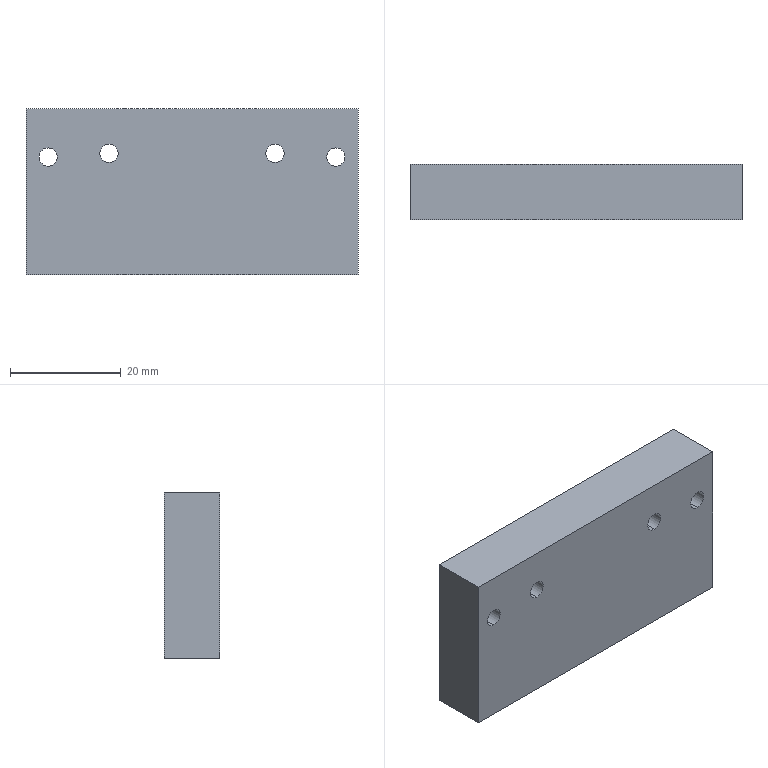Part | STEP file | 227H056123 Block_Default | 1 solid | 14 faces | box 60 x 10 x 30 mm | volume 17658 mm3 | cylinder 8 | plane 6 | commonest cylinder face diameters 3.3 x8
STEP:
#1=CARTESIAN_POINT('',(0.,0.,0.));
#2=DIRECTION('',(0.,0.,1.));
#3=DIRECTION('',(1.,0.,0.));
#4=AXIS2_PLACEMENT_3D('',#1,#2,#3);
#5=CARTESIAN_POINT('',(15.,0.,8.65));
#6=VERTEX_POINT('',#5);
#7=CARTESIAN_POINT('',(15.,10.,8.65));
#8=VERTEX_POINT('',#7);
#9=CARTESIAN_POINT('',(15.,10.,8.65));
#10=DIRECTION('',(0.,1.,0.));
#11=VECTOR('',#10,1.);
#12=LINE('',#9,#11);
#13=CARTESIAN_POINT('',(15.,10.,7.));
#14=DIRECTION('',(0.,1.,0.));
#15=DIRECTION('',(0.,0.,1.));
#16=AXIS2_PLACEMENT_3D('',#13,#14,#15);
#17=CYLINDRICAL_SURFACE('',#16,1.65);
#18=CARTESIAN_POINT('',(6.283,0.));
#19=DIRECTION('',(0.,1.));
#20=VECTOR('',#19,1.);
#21=LINE('',#18,#20);
#22=(GEOMETRIC_REPRESENTATION_CONTEXT(2)PARAMETRIC_REPRESENTATION_CONTEXT()REPRESENTATION_CONTEXT('',''));
#23=DEFINITIONAL_REPRESENTATION('',(#21),#22);
#24=PCURVE('',#17,#23);
#25=CARTESIAN_POINT('',(15.,10.,7.));
#26=DIRECTION('',(0.,1.,0.));
#27=DIRECTION('',(0.,0.,1.));
#28=AXIS2_PLACEMENT_3D('',#25,#26,#27);
#29=CYLINDRICAL_SURFACE('',#28,1.65);
#30=CARTESIAN_POINT('',(0.,0.));
#31=DIRECTION('',(0.,1.));
#32=VECTOR('',#31,1.);
#33=LINE('',#30,#32);
#34=(GEOMETRIC_REPRESENTATION_CONTEXT(2)PARAMETRIC_REPRESENTATION_CONTEXT()REPRESENTATION_CONTEXT('',''));
#35=DEFINITIONAL_REPRESENTATION('',(#33),#34);
#36=PCURVE('',#29,#35);
#37=SURFACE_CURVE('',#12,(#24,#36),.PCURVE_S1.);
#38=EDGE_CURVE('',#6,#8,#37,.T.);
#39=ORIENTED_EDGE('',*,*,#38,.T.);
#40=CARTESIAN_POINT('',(15.,10.,5.35));
#41=VERTEX_POINT('',#40);
#42=CARTESIAN_POINT('',(15.,10.,7.));
#43=DIRECTION('',(0.,1.,0.));
#44=DIRECTION('',(0.,0.,1.));
#45=AXIS2_PLACEMENT_3D('',#42,#43,#44);
#46=CIRCLE('',#45,1.65);
#47=CARTESIAN_POINT('',(0.,0.));
#48=DIRECTION('',(1.,0.));
#49=VECTOR('',#48,1.);
#50=LINE('',#47,#49);
#51=(GEOMETRIC_REPRESENTATION_CONTEXT(2)PARAMETRIC_REPRESENTATION_CONTEXT()REPRESENTATION_CONTEXT('',''));
#52=DEFINITIONAL_REPRESENTATION('',(#50),#51);
#53=PCURVE('',#17,#52);
#54=CARTESIAN_POINT('',(0.,10.,0.));
#55=DIRECTION('',(0.,1.,0.));
#56=DIRECTION('',(0.,0.,1.));
#57=AXIS2_PLACEMENT_3D('',#54,#55,#56);
#58=PLANE('',#57);
#59=CARTESIAN_POINT('',(7.,15.));
#60=DIRECTION('',(1.,0.));
#61=AXIS2_PLACEMENT_2D('',#59,#60);
#62=CIRCLE('',#61,1.65);
#63=(GEOMETRIC_REPRESENTATION_CONTEXT(2)PARAMETRIC_REPRESENTATION_CONTEXT()REPRESENTATION_CONTEXT('',''));
#64=DEFINITIONAL_REPRESENTATION('',(#62),#63);
#65=PCURVE('',#58,#64);
#66=SURFACE_CURVE('',#46,(#53,#65),.PCURVE_S1.);
#67=EDGE_CURVE('',#41,#8,#66,.T.);
#68=ORIENTED_EDGE('',*,*,#67,.F.);
#69=CARTESIAN_POINT('',(15.,0.,5.35));
#70=VERTEX_POINT('',#69);
#71=CARTESIAN_POINT('',(15.,10.,5.35));
#72=DIRECTION('',(0.,1.,0.));
#73=VECTOR('',#72,1.);
#74=LINE('',#71,#73);
#75=CARTESIAN_POINT('',(3.142,0.));
#76=DIRECTION('',(0.,1.));
#77=VECTOR('',#76,1.);
#78=LINE('',#75,#77);
#79=(GEOMETRIC_REPRESENTATION_CONTEXT(2)PARAMETRIC_REPRESENTATION_CONTEXT()REPRESENTATION_CONTEXT('',''));
#80=DEFINITIONAL_REPRESENTATION('',(#78),#79);
#81=PCURVE('',#17,#80);
#82=CARTESIAN_POINT('',(3.142,0.));
#83=DIRECTION('',(0.,1.));
#84=VECTOR('',#83,1.);
#85=LINE('',#82,#84);
#86=(GEOMETRIC_REPRESENTATION_CONTEXT(2)PARAMETRIC_REPRESENTATION_CONTEXT()REPRESENTATION_CONTEXT('',''));
#87=DEFINITIONAL_REPRESENTATION('',(#85),#86);
#88=PCURVE('',#29,#87);
#89=SURFACE_CURVE('',#74,(#81,#88),.PCURVE_S1.);
#90=EDGE_CURVE('',#70,#41,#89,.T.);
#91=ORIENTED_EDGE('',*,*,#90,.F.);
#92=CARTESIAN_POINT('',(15.,0.,7.));
#93=DIRECTION('',(0.,1.,0.));
#94=DIRECTION('',(0.,0.,1.));
#95=AXIS2_PLACEMENT_3D('',#92,#93,#94);
#96=CIRCLE('',#95,1.65);
#97=CARTESIAN_POINT('',(0.,-10.));
#98=DIRECTION('',(1.,0.));
#99=VECTOR('',#98,1.);
#100=LINE('',#97,#99);
#101=(GEOMETRIC_REPRESENTATION_CONTEXT(2)PARAMETRIC_REPRESENTATION_CONTEXT()REPRESENTATION_CONTEXT('',''));
#102=DEFINITIONAL_REPRESENTATION('',(#100),#101);
#103=PCURVE('',#17,#102);
#104=CARTESIAN_POINT('',(0.,0.,0.));
#105=DIRECTION('',(0.,1.,0.));
#106=DIRECTION('',(0.,0.,1.));
#107=AXIS2_PLACEMENT_3D('',#104,#105,#106);
#108=PLANE('',#107);
#109=CARTESIAN_POINT('',(7.,15.));
#110=DIRECTION('',(1.,0.));
#111=AXIS2_PLACEMENT_2D('',#109,#110);
#112=CIRCLE('',#111,1.65);
#113=(GEOMETRIC_REPRESENTATION_CONTEXT(2)PARAMETRIC_REPRESENTATION_CONTEXT()REPRESENTATION_CONTEXT('',''));
#114=DEFINITIONAL_REPRESENTATION('',(#112),#113);
#115=PCURVE('',#108,#114);
#116=SURFACE_CURVE('',#96,(#103,#115),.PCURVE_S1.);
#117=EDGE_CURVE('',#70,#6,#116,.T.);
#118=ORIENTED_EDGE('',*,*,#117,.T.);
#119=EDGE_LOOP('',(#39,#68,#91,#118));
#120=FACE_BOUND('',#119,.F.);
#121=ADVANCED_FACE('',(#120),#17,.F.);
#122=CARTESIAN_POINT('',(-15.,0.,8.65));
#123=VERTEX_POINT('',#122);
#124=CARTESIAN_POINT('',(-15.,10.,8.65));
#125=VERTEX_POINT('',#124);
#126=CARTESIAN_POINT('',(-15.,10.,8.65));
#127=DIRECTION('',(0.,1.,0.));
#128=VECTOR('',#127,1.);
#129=LINE('',#126,#128);
#130=CARTESIAN_POINT('',(-15.,10.,7.));
#131=DIRECTION('',(0.,1.,0.));
#132=DIRECTION('',(0.,0.,1.));
#133=AXIS2_PLACEMENT_3D('',#130,#131,#132);
#134=CYLINDRICAL_SURFACE('',#133,1.65);
#135=CARTESIAN_POINT('',(6.283,0.));
#136=DIRECTION('',(0.,1.));
#137=VECTOR('',#136,1.);
#138=LINE('',#135,#137);
#139=(GEOMETRIC_REPRESENTATION_CONTEXT(2)PARAMETRIC_REPRESENTATION_CONTEXT()REPRESENTATION_CONTEXT('',''));
#140=DEFINITIONAL_REPRESENTATION('',(#138),#139);
#141=PCURVE('',#134,#140);
#142=CARTESIAN_POINT('',(-15.,10.,7.));
#143=DIRECTION('',(0.,1.,0.));
#144=DIRECTION('',(0.,0.,1.));
#145=AXIS2_PLACEMENT_3D('',#142,#143,#144);
#146=CYLINDRICAL_SURFACE('',#145,1.65);
#147=CARTESIAN_POINT('',(0.,0.));
#148=DIRECTION('',(0.,1.));
#149=VECTOR('',#148,1.);
#150=LINE('',#147,#149);
#151=(GEOMETRIC_REPRESENTATION_CONTEXT(2)PARAMETRIC_REPRESENTATION_CONTEXT()REPRESENTATION_CONTEXT('',''));
#152=DEFINITIONAL_REPRESENTATION('',(#150),#151);
#153=PCURVE('',#146,#152);
#154=SURFACE_CURVE('',#129,(#141,#153),.PCURVE_S1.);
#155=EDGE_CURVE('',#123,#125,#154,.T.);
#156=ORIENTED_EDGE('',*,*,#155,.T.);
#157=CARTESIAN_POINT('',(-15.,10.,5.35));
#158=VERTEX_POINT('',#157);
#159=CARTESIAN_POINT('',(-15.,10.,7.));
#160=DIRECTION('',(0.,1.,0.));
#161=DIRECTION('',(0.,0.,1.));
#162=AXIS2_PLACEMENT_3D('',#159,#160,#161);
#163=CIRCLE('',#162,1.65);
#164=CARTESIAN_POINT('',(0.,0.));
#165=DIRECTION('',(1.,0.));
#166=VECTOR('',#165,1.);
#167=LINE('',#164,#166);
#168=(GEOMETRIC_REPRESENTATION_CONTEXT(2)PARAMETRIC_REPRESENTATION_CONTEXT()REPRESENTATION_CONTEXT('',''));
#169=DEFINITIONAL_REPRESENTATION('',(#167),#168);
#170=PCURVE('',#134,#169);
#171=CARTESIAN_POINT('',(7.,-15.));
#172=DIRECTION('',(1.,0.));
#173=AXIS2_PLACEMENT_2D('',#171,#172);
#174=CIRCLE('',#173,1.65);
#175=(GEOMETRIC_REPRESENTATION_CONTEXT(2)PARAMETRIC_REPRESENTATION_CONTEXT()REPRESENTATION_CONTEXT('',''));
#176=DEFINITIONAL_REPRESENTATION('',(#174),#175);
#177=PCURVE('',#58,#176);
#178=SURFACE_CURVE('',#163,(#170,#177),.PCURVE_S1.);
#179=EDGE_CURVE('',#158,#125,#178,.T.);
#180=ORIENTED_EDGE('',*,*,#179,.F.);
#181=CARTESIAN_POINT('',(-15.,0.,5.35));
#182=VERTEX_POINT('',#181);
#183=CARTESIAN_POINT('',(-15.,10.,5.35));
#184=DIRECTION('',(0.,1.,0.));
#185=VECTOR('',#184,1.);
#186=LINE('',#183,#185);
#187=CARTESIAN_POINT('',(3.142,0.));
#188=DIRECTION('',(0.,1.));
#189=VECTOR('',#188,1.);
#190=LINE('',#187,#189);
#191=(GEOMETRIC_REPRESENTATION_CONTEXT(2)PARAMETRIC_REPRESENTATION_CONTEXT()REPRESENTATION_CONTEXT('',''));
#192=DEFINITIONAL_REPRESENTATION('',(#190),#191);
#193=PCURVE('',#134,#192);
#194=CARTESIAN_POINT('',(3.142,0.));
#195=DIRECTION('',(0.,1.));
#196=VECTOR('',#195,1.);
#197=LINE('',#194,#196);
#198=(GEOMETRIC_REPRESENTATION_CONTEXT(2)PARAMETRIC_REPRESENTATION_CONTEXT()REPRESENTATION_CONTEXT('',''));
#199=DEFINITIONAL_REPRESENTATION('',(#197),#198);
#200=PCURVE('',#146,#199);
#201=SURFACE_CURVE('',#186,(#193,#200),.PCURVE_S1.);
#202=EDGE_CURVE('',#182,#158,#201,.T.);
#203=ORIENTED_EDGE('',*,*,#202,.F.);
#204=CARTESIAN_POINT('',(-15.,0.,7.));
#205=DIRECTION('',(0.,1.,0.));
#206=DIRECTION('',(0.,0.,1.));
#207=AXIS2_PLACEMENT_3D('',#204,#205,#206);
#208=CIRCLE('',#207,1.65);
#209=CARTESIAN_POINT('',(0.,-10.));
#210=DIRECTION('',(1.,0.));
#211=VECTOR('',#210,1.);
#212=LINE('',#209,#211);
#213=(GEOMETRIC_REPRESENTATION_CONTEXT(2)PARAMETRIC_REPRESENTATION_CONTEXT()REPRESENTATION_CONTEXT('',''));
#214=DEFINITIONAL_REPRESENTATION('',(#212),#213);
#215=PCURVE('',#134,#214);
#216=CARTESIAN_POINT('',(7.,-15.));
#217=DIRECTION('',(1.,0.));
#218=AXIS2_PLACEMENT_2D('',#216,#217);
#219=CIRCLE('',#218,1.65);
#220=(GEOMETRIC_REPRESENTATION_CONTEXT(2)PARAMETRIC_REPRESENTATION_CONTEXT()REPRESENTATION_CONTEXT('',''));
#221=DEFINITIONAL_REPRESENTATION('',(#219),#220);
#222=PCURVE('',#108,#221);
#223=SURFACE_CURVE('',#208,(#215,#222),.PCURVE_S1.);
#224=EDGE_CURVE('',#182,#123,#223,.T.);
#225=ORIENTED_EDGE('',*,*,#224,.T.);
#226=EDGE_LOOP('',(#156,#180,#203,#225));
#227=FACE_BOUND('',#226,.F.);
#228=ADVANCED_FACE('',(#227),#134,.F.);
#229=CARTESIAN_POINT('',(26.,10.,4.661));
#230=VERTEX_POINT('',#229);
#231=CARTESIAN_POINT('',(26.,0.,4.661));
#232=VERTEX_POINT('',#231);
#233=CARTESIAN_POINT('',(26.,0.,4.661));
#234=DIRECTION('',(0.,-1.,0.));
#235=VECTOR('',#234,1.);
#236=LINE('',#233,#235);
#237=CARTESIAN_POINT('',(26.,0.,6.311));
#238=DIRECTION('',(0.,-1.,0.));
#239=DIRECTION('',(0.,0.,-1.));
#240=AXIS2_PLACEMENT_3D('',#237,#238,#239);
#241=CYLINDRICAL_SURFACE('',#240,1.65);
#242=CARTESIAN_POINT('',(6.283,0.));
#243=DIRECTION('',(0.,1.));
#244=VECTOR('',#243,1.);
#245=LINE('',#242,#244);
#246=(GEOMETRIC_REPRESENTATION_CONTEXT(2)PARAMETRIC_REPRESENTATION_CONTEXT()REPRESENTATION_CONTEXT('',''));
#247=DEFINITIONAL_REPRESENTATION('',(#245),#246);
#248=PCURVE('',#241,#247);
#249=CARTESIAN_POINT('',(26.,0.,6.311));
#250=DIRECTION('',(0.,-1.,0.));
#251=DIRECTION('',(0.,0.,-1.));
#252=AXIS2_PLACEMENT_3D('',#249,#250,#251);
#253=CYLINDRICAL_SURFACE('',#252,1.65);
#254=CARTESIAN_POINT('',(0.,0.));
#255=DIRECTION('',(0.,1.));
#256=VECTOR('',#255,1.);
#257=LINE('',#254,#256);
#258=(GEOMETRIC_REPRESENTATION_CONTEXT(2)PARAMETRIC_REPRESENTATION_CONTEXT()REPRESENTATION_CONTEXT('',''));
#259=DEFINITIONAL_REPRESENTATION('',(#257),#258);
#260=PCURVE('',#253,#259);
#261=SURFACE_CURVE('',#236,(#248,#260),.PCURVE_S1.);
#262=EDGE_CURVE('',#230,#232,#261,.T.);
#263=ORIENTED_EDGE('',*,*,#262,.T.);
#264=CARTESIAN_POINT('',(26.,0.,7.961));
#265=VERTEX_POINT('',#264);
#266=CARTESIAN_POINT('',(26.,0.,6.311));
#267=DIRECTION('',(0.,-1.,0.));
#268=DIRECTION('',(0.,0.,-1.));
#269=AXIS2_PLACEMENT_3D('',#266,#267,#268);
#270=CIRCLE('',#269,1.65);
#271=CARTESIAN_POINT('',(0.,0.));
#272=DIRECTION('',(1.,0.));
#273=VECTOR('',#272,1.);
#274=LINE('',#271,#273);
#275=(GEOMETRIC_REPRESENTATION_CONTEXT(2)PARAMETRIC_REPRESENTATION_CONTEXT()REPRESENTATION_CONTEXT('',''));
#276=DEFINITIONAL_REPRESENTATION('',(#274),#275);
#277=PCURVE('',#241,#276);
#278=CARTESIAN_POINT('',(4.661,26.));
#279=CARTESIAN_POINT('',(4.661,28.858));
#280=CARTESIAN_POINT('',(7.136,27.429));
#281=CARTESIAN_POINT('',(9.611,26.));
#282=CARTESIAN_POINT('',(7.136,24.571));
#283=CARTESIAN_POINT('',(4.661,23.142));
#284=CARTESIAN_POINT('',(4.661,26.));
#285=(BOUNDED_CURVE()B_SPLINE_CURVE(2,(#278,#279,#280,#281,#282,#283,#284),.UNSPECIFIED.,.T.,.F.)B_SPLINE_CURVE_WITH_KNOTS((1,2,2,2,2,1),(-2.094,0.,2.094,4.189,6.283,8.378),.UNSPECIFIED.)CURVE()GEOMETRIC_REPRESENTATION_ITEM()RATIONAL_B_SPLINE_CURVE((1.,0.5,1.,0.5,1.,0.5,1.))REPRESENTATION_ITEM(''));
#286=(GEOMETRIC_REPRESENTATION_CONTEXT(2)PARAMETRIC_REPRESENTATION_CONTEXT()REPRESENTATION_CONTEXT('',''));
#287=DEFINITIONAL_REPRESENTATION('',(#285),#286);
#288=PCURVE('',#108,#287);
#289=SURFACE_CURVE('',#270,(#277,#288),.PCURVE_S1.);
#290=EDGE_CURVE('',#265,#232,#289,.T.);
#291=ORIENTED_EDGE('',*,*,#290,.F.);
#292=CARTESIAN_POINT('',(26.,10.,7.961));
#293=VERTEX_POINT('',#292);
#294=CARTESIAN_POINT('',(26.,0.,7.961));
#295=DIRECTION('',(0.,-1.,0.));
#296=VECTOR('',#295,1.);
#297=LINE('',#294,#296);
#298=CARTESIAN_POINT('',(3.142,0.));
#299=DIRECTION('',(0.,1.));
#300=VECTOR('',#299,1.);
#301=LINE('',#298,#300);
#302=(GEOMETRIC_REPRESENTATION_CONTEXT(2)PARAMETRIC_REPRESENTATION_CONTEXT()REPRESENTATION_CONTEXT('',''));
#303=DEFINITIONAL_REPRESENTATION('',(#301),#302);
#304=PCURVE('',#241,#303);
#305=CARTESIAN_POINT('',(3.142,0.));
#306=DIRECTION('',(0.,1.));
#307=VECTOR('',#306,1.);
#308=LINE('',#305,#307);
#309=(GEOMETRIC_REPRESENTATION_CONTEXT(2)PARAMETRIC_REPRESENTATION_CONTEXT()REPRESENTATION_CONTEXT('',''));
#310=DEFINITIONAL_REPRESENTATION('',(#308),#309);
#311=PCURVE('',#253,#310);
#312=SURFACE_CURVE('',#297,(#304,#311),.PCURVE_S1.);
#313=EDGE_CURVE('',#293,#265,#312,.T.);
#314=ORIENTED_EDGE('',*,*,#313,.F.);
#315=CARTESIAN_POINT('',(26.,10.,6.311));
#316=DIRECTION('',(0.,-1.,0.));
#317=DIRECTION('',(0.,0.,-1.));
#318=AXIS2_PLACEMENT_3D('',#315,#316,#317);
#319=CIRCLE('',#318,1.65);
#320=CARTESIAN_POINT('',(0.,-10.));
#321=DIRECTION('',(1.,0.));
#322=VECTOR('',#321,1.);
#323=LINE('',#320,#322);
#324=(GEOMETRIC_REPRESENTATION_CONTEXT(2)PARAMETRIC_REPRESENTATION_CONTEXT()REPRESENTATION_CONTEXT('',''));
#325=DEFINITIONAL_REPRESENTATION('',(#323),#324);
#326=PCURVE('',#241,#325);
#327=CARTESIAN_POINT('',(4.661,26.));
#328=CARTESIAN_POINT('',(4.661,28.858));
#329=CARTESIAN_POINT('',(7.136,27.429));
#330=CARTESIAN_POINT('',(9.611,26.));
#331=CARTESIAN_POINT('',(7.136,24.571));
#332=CARTESIAN_POINT('',(4.661,23.142));
#333=CARTESIAN_POINT('',(4.661,26.));
#334=(BOUNDED_CURVE()B_SPLINE_CURVE(2,(#327,#328,#329,#330,#331,#332,#333),.UNSPECIFIED.,.T.,.F.)B_SPLINE_CURVE_WITH_KNOTS((1,2,2,2,2,1),(-2.094,0.,2.094,4.189,6.283,8.378),.UNSPECIFIED.)CURVE()GEOMETRIC_REPRESENTATION_ITEM()RATIONAL_B_SPLINE_CURVE((1.,0.5,1.,0.5,1.,0.5,1.))REPRESENTATION_ITEM(''));
#335=(GEOMETRIC_REPRESENTATION_CONTEXT(2)PARAMETRIC_REPRESENTATION_CONTEXT()REPRESENTATION_CONTEXT('',''));
#336=DEFINITIONAL_REPRESENTATION('',(#334),#335);
#337=PCURVE('',#58,#336);
#338=SURFACE_CURVE('',#319,(#326,#337),.PCURVE_S1.);
#339=EDGE_CURVE('',#293,#230,#338,.T.);
#340=ORIENTED_EDGE('',*,*,#339,.T.);
#341=EDGE_LOOP('',(#263,#291,#314,#340));
#342=FACE_BOUND('',#341,.F.);
#343=ADVANCED_FACE('',(#342),#241,.F.);
#344=CARTESIAN_POINT('',(-26.,10.,4.661));
#345=VERTEX_POINT('',#344);
#346=CARTESIAN_POINT('',(-26.,0.,4.661));
#347=VERTEX_POINT('',#346);
#348=CARTESIAN_POINT('',(-26.,0.,4.661));
#349=DIRECTION('',(0.,-1.,0.));
#350=VECTOR('',#349,1.);
#351=LINE('',#348,#350);
#352=CARTESIAN_POINT('',(-26.,0.,6.311));
#353=DIRECTION('',(0.,-1.,0.));
#354=DIRECTION('',(0.,0.,-1.));
#355=AXIS2_PLACEMENT_3D('',#352,#353,#354);
#356=CYLINDRICAL_SURFACE('',#355,1.65);
#357=CARTESIAN_POINT('',(6.283,0.));
#358=DIRECTION('',(0.,1.));
#359=VECTOR('',#358,1.);
#360=LINE('',#357,#359);
#361=(GEOMETRIC_REPRESENTATION_CONTEXT(2)PARAMETRIC_REPRESENTATION_CONTEXT()REPRESENTATION_CONTEXT('',''));
#362=DEFINITIONAL_REPRESENTATION('',(#360),#361);
#363=PCURVE('',#356,#362);
#364=CARTESIAN_POINT('',(-26.,0.,6.311));
#365=DIRECTION('',(0.,-1.,0.));
#366=DIRECTION('',(0.,0.,-1.));
#367=AXIS2_PLACEMENT_3D('',#364,#365,#366);
#368=CYLINDRICAL_SURFACE('',#367,1.65);
#369=CARTESIAN_POINT('',(0.,0.));
#370=DIRECTION('',(0.,1.));
#371=VECTOR('',#370,1.);
#372=LINE('',#369,#371);
#373=(GEOMETRIC_REPRESENTATION_CONTEXT(2)PARAMETRIC_REPRESENTATION_CONTEXT()REPRESENTATION_CONTEXT('',''));
#374=DEFINITIONAL_REPRESENTATION('',(#372),#373);
#375=PCURVE('',#368,#374);
#376=SURFACE_CURVE('',#351,(#363,#375),.PCURVE_S1.);
#377=EDGE_CURVE('',#345,#347,#376,.T.);
#378=ORIENTED_EDGE('',*,*,#377,.T.);
#379=CARTESIAN_POINT('',(-26.,0.,7.961));
#380=VERTEX_POINT('',#379);
#381=CARTESIAN_POINT('',(-26.,0.,6.311));
#382=DIRECTION('',(0.,-1.,0.));
#383=DIRECTION('',(0.,0.,-1.));
#384=AXIS2_PLACEMENT_3D('',#381,#382,#383);
#385=CIRCLE('',#384,1.65);
#386=CARTESIAN_POINT('',(0.,0.));
#387=DIRECTION('',(1.,0.));
#388=VECTOR('',#387,1.);
#389=LINE('',#386,#388);
#390=(GEOMETRIC_REPRESENTATION_CONTEXT(2)PARAMETRIC_REPRESENTATION_CONTEXT()REPRESENTATION_CONTEXT('',''));
#391=DEFINITIONAL_REPRESENTATION('',(#389),#390);
#392=PCURVE('',#356,#391);
#393=CARTESIAN_POINT('',(4.661,-26.));
#394=CARTESIAN_POINT('',(4.661,-23.142));
#395=CARTESIAN_POINT('',(7.136,-24.571));
#396=CARTESIAN_POINT('',(9.611,-26.));
#397=CARTESIAN_POINT('',(7.136,-27.429));
#398=CARTESIAN_POINT('',(4.661,-28.858));
#399=CARTESIAN_POINT('',(4.661,-26.));
#400=(BOUNDED_CURVE()B_SPLINE_CURVE(2,(#393,#394,#395,#396,#397,#398,#399),.UNSPECIFIED.,.T.,.F.)B_SPLINE_CURVE_WITH_KNOTS((1,2,2,2,2,1),(-2.094,0.,2.094,4.189,6.283,8.378),.UNSPECIFIED.)CURVE()GEOMETRIC_REPRESENTATION_ITEM()RATIONAL_B_SPLINE_CURVE((1.,0.5,1.,0.5,1.,0.5,1.))REPRESENTATION_ITEM(''));
#401=(GEOMETRIC_REPRESENTATION_CONTEXT(2)PARAMETRIC_REPRESENTATION_CONTEXT()REPRESENTATION_CONTEXT('',''));
#402=DEFINITIONAL_REPRESENTATION('',(#400),#401);
#403=PCURVE('',#108,#402);
#404=SURFACE_CURVE('',#385,(#392,#403),.PCURVE_S1.);
#405=EDGE_CURVE('',#380,#347,#404,.T.);
#406=ORIENTED_EDGE('',*,*,#405,.F.);
#407=CARTESIAN_POINT('',(-26.,10.,7.961));
#408=VERTEX_POINT('',#407);
#409=CARTESIAN_POINT('',(-26.,0.,7.961));
#410=DIRECTION('',(0.,-1.,0.));
#411=VECTOR('',#410,1.);
#412=LINE('',#409,#411);
#413=CARTESIAN_POINT('',(3.142,0.));
#414=DIRECTION('',(0.,1.));
#415=VECTOR('',#414,1.);
#416=LINE('',#413,#415);
#417=(GEOMETRIC_REPRESENTATION_CONTEXT(2)PARAMETRIC_REPRESENTATION_CONTEXT()REPRESENTATION_CONTEXT('',''));
#418=DEFINITIONAL_REPRESENTATION('',(#416),#417);
#419=PCURVE('',#356,#418);
#420=CARTESIAN_POINT('',(3.142,0.));
#421=DIRECTION('',(0.,1.));
#422=VECTOR('',#421,1.);
#423=LINE('',#420,#422);
#424=(GEOMETRIC_REPRESENTATION_CONTEXT(2)PARAMETRIC_REPRESENTATION_CONTEXT()REPRESENTATION_CONTEXT('',''));
#425=DEFINITIONAL_REPRESENTATION('',(#423),#424);
#426=PCURVE('',#368,#425);
#427=SURFACE_CURVE('',#412,(#419,#426),.PCURVE_S1.);
#428=EDGE_CURVE('',#408,#380,#427,.T.);
#429=ORIENTED_EDGE('',*,*,#428,.F.);
#430=CARTESIAN_POINT('',(-26.,10.,6.311));
#431=DIRECTION('',(0.,-1.,0.));
#432=DIRECTION('',(0.,0.,-1.));
#433=AXIS2_PLACEMENT_3D('',#430,#431,#432);
#434=CIRCLE('',#433,1.65);
#435=CARTESIAN_POINT('',(0.,-10.));
#436=DIRECTION('',(1.,0.));
#437=VECTOR('',#436,1.);
#438=LINE('',#435,#437);
#439=(GEOMETRIC_REPRESENTATION_CONTEXT(2)PARAMETRIC_REPRESENTATION_CONTEXT()REPRESENTATION_CONTEXT('',''));
#440=DEFINITIONAL_REPRESENTATION('',(#438),#439);
#441=PCURVE('',#356,#440);
#442=CARTESIAN_POINT('',(4.661,-26.));
#443=CARTESIAN_POINT('',(4.661,-23.142));
#444=CARTESIAN_POINT('',(7.136,-24.571));
#445=CARTESIAN_POINT('',(9.611,-26.));
#446=CARTESIAN_POINT('',(7.136,-27.429));
#447=CARTESIAN_POINT('',(4.661,-28.858));
#448=CARTESIAN_POINT('',(4.661,-26.));
#449=(BOUNDED_CURVE()B_SPLINE_CURVE(2,(#442,#443,#444,#445,#446,#447,#448),.UNSPECIFIED.,.T.,.F.)B_SPLINE_CURVE_WITH_KNOTS((1,2,2,2,2,1),(-2.094,0.,2.094,4.189,6.283,8.378),.UNSPECIFIED.)CURVE()GEOMETRIC_REPRESENTATION_ITEM()RATIONAL_B_SPLINE_CURVE((1.,0.5,1.,0.5,1.,0.5,1.))REPRESENTATION_ITEM(''));
#450=(GEOMETRIC_REPRESENTATION_CONTEXT(2)PARAMETRIC_REPRESENTATION_CONTEXT()REPRESENTATION_CONTEXT('',''));
#451=DEFINITIONAL_REPRESENTATION('',(#449),#450);
#452=PCURVE('',#58,#451);
#453=SURFACE_CURVE('',#434,(#441,#452),.PCURVE_S1.);
#454=EDGE_CURVE('',#408,#345,#453,.T.);
#455=ORIENTED_EDGE('',*,*,#454,.T.);
#456=EDGE_LOOP('',(#378,#406,#429,#455));
#457=FACE_BOUND('',#456,.F.);
#458=ADVANCED_FACE('',(#457),#356,.F.);
#459=CARTESIAN_POINT('',(-30.,0.,-15.));
#460=VERTEX_POINT('',#459);
#461=CARTESIAN_POINT('',(-30.,0.,15.));
#462=VERTEX_POINT('',#461);
#463=CARTESIAN_POINT('',(-30.,0.,15.));
#464=DIRECTION('',(0.,0.,1.));
#465=VECTOR('',#464,1.);
#466=LINE('',#463,#465);
#467=CARTESIAN_POINT('',(-30.,10.,15.));
#468=DIRECTION('',(1.,0.,0.));
#469=DIRECTION('',(0.,0.,-1.));
#470=AXIS2_PLACEMENT_3D('',#467,#468,#469);
#471=PLANE('',#470);
#472=CARTESIAN_POINT('',(0.,-10.));
#473=DIRECTION('',(-1.,0.));
#474=VECTOR('',#473,1.);
#475=LINE('',#472,#474);
#476=(GEOMETRIC_REPRESENTATION_CONTEXT(2)PARAMETRIC_REPRESENTATION_CONTEXT()REPRESENTATION_CONTEXT('',''));
#477=DEFINITIONAL_REPRESENTATION('',(#475),#476);
#478=PCURVE('',#471,#477);
#479=CARTESIAN_POINT('',(15.,-30.));
#480=DIRECTION('',(1.,0.));
#481=VECTOR('',#480,1.);
#482=LINE('',#479,#481);
#483=(GEOMETRIC_REPRESENTATION_CONTEXT(2)PARAMETRIC_REPRESENTATION_CONTEXT()REPRESENTATION_CONTEXT('',''));
#484=DEFINITIONAL_REPRESENTATION('',(#482),#483);
#485=PCURVE('',#108,#484);
#486=SURFACE_CURVE('',#466,(#478,#485),.PCURVE_S1.);
#487=EDGE_CURVE('',#460,#462,#486,.T.);
#488=ORIENTED_EDGE('',*,*,#487,.T.);
#489=CARTESIAN_POINT('',(-30.,10.,15.));
#490=VERTEX_POINT('',#489);
#491=CARTESIAN_POINT('',(-30.,10.,15.));
#492=DIRECTION('',(0.,-1.,0.));
#493=VECTOR('',#492,1.);
#494=LINE('',#491,#493);
#495=CARTESIAN_POINT('',(0.,0.));
#496=DIRECTION('',(0.,-1.));
#497=VECTOR('',#496,1.);
#498=LINE('',#495,#497);
#499=(GEOMETRIC_REPRESENTATION_CONTEXT(2)PARAMETRIC_REPRESENTATION_CONTEXT()REPRESENTATION_CONTEXT('',''));
#500=DEFINITIONAL_REPRESENTATION('',(#498),#499);
#501=PCURVE('',#471,#500);
#502=CARTESIAN_POINT('',(30.,10.,15.));
#503=DIRECTION('',(0.,0.,-1.));
#504=DIRECTION('',(-1.,0.,0.));
#505=AXIS2_PLACEMENT_3D('',#502,#503,#504);
#506=PLANE('',#505);
#507=CARTESIAN_POINT('',(60.,0.));
#508=DIRECTION('',(0.,-1.));
#509=VECTOR('',#508,1.);
#510=LINE('',#507,#509);
#511=(GEOMETRIC_REPRESENTATION_CONTEXT(2)PARAMETRIC_REPRESENTATION_CONTEXT()REPRESENTATION_CONTEXT('',''));
#512=DEFINITIONAL_REPRESENTATION('',(#510),#511);
#513=PCURVE('',#506,#512);
#514=SURFACE_CURVE('',#494,(#501,#513),.PCURVE_S1.);
#515=EDGE_CURVE('',#490,#462,#514,.T.);
#516=ORIENTED_EDGE('',*,*,#515,.F.);
#517=CARTESIAN_POINT('',(-30.,10.,-15.));
#518=VERTEX_POINT('',#517);
#519=CARTESIAN_POINT('',(-30.,10.,15.));
#520=DIRECTION('',(0.,0.,1.));
#521=VECTOR('',#520,1.);
#522=LINE('',#519,#521);
#523=CARTESIAN_POINT('',(0.,0.));
#524=DIRECTION('',(-1.,0.));
#525=VECTOR('',#524,1.);
#526=LINE('',#523,#525);
#527=(GEOMETRIC_REPRESENTATION_CONTEXT(2)PARAMETRIC_REPRESENTATION_CONTEXT()REPRESENTATION_CONTEXT('',''));
#528=DEFINITIONAL_REPRESENTATION('',(#526),#527);
#529=PCURVE('',#471,#528);
#530=CARTESIAN_POINT('',(15.,-30.));
#531=DIRECTION('',(1.,0.));
#532=VECTOR('',#531,1.);
#533=LINE('',#530,#532);
#534=(GEOMETRIC_REPRESENTATION_CONTEXT(2)PARAMETRIC_REPRESENTATION_CONTEXT()REPRESENTATION_CONTEXT('',''));
#535=DEFINITIONAL_REPRESENTATION('',(#533),#534);
#536=PCURVE('',#58,#535);
#537=SURFACE_CURVE('',#522,(#529,#536),.PCURVE_S1.);
#538=EDGE_CURVE('',#518,#490,#537,.T.);
#539=ORIENTED_EDGE('',*,*,#538,.F.);
#540=CARTESIAN_POINT('',(-30.,10.,-15.));
#541=DIRECTION('',(0.,-1.,0.));
#542=VECTOR('',#541,1.);
#543=LINE('',#540,#542);
#544=CARTESIAN_POINT('',(30.,0.));
#545=DIRECTION('',(0.,-1.));
#546=VECTOR('',#545,1.);
#547=LINE('',#544,#546);
#548=(GEOMETRIC_REPRESENTATION_CONTEXT(2)PARAMETRIC_REPRESENTATION_CONTEXT()REPRESENTATION_CONTEXT('',''));
#549=DEFINITIONAL_REPRESENTATION('',(#547),#548);
#550=PCURVE('',#471,#549);
#551=CARTESIAN_POINT('',(30.,10.,-15.));
#552=DIRECTION('',(0.,0.,1.));
#553=DIRECTION('',(1.,0.,0.));
#554=AXIS2_PLACEMENT_3D('',#551,#552,#553);
#555=PLANE('',#554);
#556=CARTESIAN_POINT('',(-60.,0.));
#557=DIRECTION('',(0.,-1.));
#558=VECTOR('',#557,1.);
#559=LINE('',#556,#558);
#560=(GEOMETRIC_REPRESENTATION_CONTEXT(2)PARAMETRIC_REPRESENTATION_CONTEXT()REPRESENTATION_CONTEXT('',''));
#561=DEFINITIONAL_REPRESENTATION('',(#559),#560);
#562=PCURVE('',#555,#561);
#563=SURFACE_CURVE('',#543,(#550,#562),.PCURVE_S1.);
#564=EDGE_CURVE('',#518,#460,#563,.T.);
#565=ORIENTED_EDGE('',*,*,#564,.T.);
#566=EDGE_LOOP('',(#488,#516,#539,#565));
#567=FACE_BOUND('',#566,.T.);
#568=ADVANCED_FACE('',(#567),#471,.F.);
#569=CARTESIAN_POINT('',(30.,0.,15.));
#570=VERTEX_POINT('',#569);
#571=CARTESIAN_POINT('',(30.,0.,15.));
#572=DIRECTION('',(1.,0.,0.));
#573=VECTOR('',#572,1.);
#574=LINE('',#571,#573);
#575=CARTESIAN_POINT('',(0.,-10.));
#576=DIRECTION('',(-1.,0.));
#577=VECTOR('',#576,1.);
#578=LINE('',#575,#577);
#579=(GEOMETRIC_REPRESENTATION_CONTEXT(2)PARAMETRIC_REPRESENTATION_CONTEXT()REPRESENTATION_CONTEXT('',''));
#580=DEFINITIONAL_REPRESENTATION('',(#578),#579);
#581=PCURVE('',#506,#580);
#582=CARTESIAN_POINT('',(15.,30.));
#583=DIRECTION('',(0.,1.));
#584=VECTOR('',#583,1.);
#585=LINE('',#582,#584);
#586=(GEOMETRIC_REPRESENTATION_CONTEXT(2)PARAMETRIC_REPRESENTATION_CONTEXT()REPRESENTATION_CONTEXT('',''));
#587=DEFINITIONAL_REPRESENTATION('',(#585),#586);
#588=PCURVE('',#108,#587);
#589=SURFACE_CURVE('',#574,(#581,#588),.PCURVE_S1.);
#590=EDGE_CURVE('',#462,#570,#589,.T.);
#591=ORIENTED_EDGE('',*,*,#590,.T.);
#592=CARTESIAN_POINT('',(30.,10.,15.));
#593=VERTEX_POINT('',#592);
#594=CARTESIAN_POINT('',(30.,10.,15.));
#595=DIRECTION('',(0.,-1.,0.));
#596=VECTOR('',#595,1.);
#597=LINE('',#594,#596);
#598=CARTESIAN_POINT('',(0.,0.));
#599=DIRECTION('',(0.,-1.));
#600=VECTOR('',#599,1.);
#601=LINE('',#598,#600);
#602=(GEOMETRIC_REPRESENTATION_CONTEXT(2)PARAMETRIC_REPRESENTATION_CONTEXT()REPRESENTATION_CONTEXT('',''));
#603=DEFINITIONAL_REPRESENTATION('',(#601),#602);
#604=PCURVE('',#506,#603);
#605=CARTESIAN_POINT('',(30.,10.,15.));
#606=DIRECTION('',(-1.,0.,0.));
#607=DIRECTION('',(0.,0.,1.));
#608=AXIS2_PLACEMENT_3D('',#605,#606,#607);
#609=PLANE('',#608);
#610=CARTESIAN_POINT('',(0.,0.));
#611=DIRECTION('',(0.,-1.));
#612=VECTOR('',#611,1.);
#613=LINE('',#610,#612);
#614=(GEOMETRIC_REPRESENTATION_CONTEXT(2)PARAMETRIC_REPRESENTATION_CONTEXT()REPRESENTATION_CONTEXT('',''));
#615=DEFINITIONAL_REPRESENTATION('',(#613),#614);
#616=PCURVE('',#609,#615);
#617=SURFACE_CURVE('',#597,(#604,#616),.PCURVE_S1.);
#618=EDGE_CURVE('',#593,#570,#617,.T.);
#619=ORIENTED_EDGE('',*,*,#618,.F.);
#620=CARTESIAN_POINT('',(30.,10.,15.));
#621=DIRECTION('',(1.,0.,0.));
#622=VECTOR('',#621,1.);
#623=LINE('',#620,#622);
#624=CARTESIAN_POINT('',(0.,0.));
#625=DIRECTION('',(-1.,0.));
#626=VECTOR('',#625,1.);
#627=LINE('',#624,#626);
#628=(GEOMETRIC_REPRESENTATION_CONTEXT(2)PARAMETRIC_REPRESENTATION_CONTEXT()REPRESENTATION_CONTEXT('',''));
#629=DEFINITIONAL_REPRESENTATION('',(#627),#628);
#630=PCURVE('',#506,#629);
#631=CARTESIAN_POINT('',(15.,30.));
#632=DIRECTION('',(0.,1.));
#633=VECTOR('',#632,1.);
#634=LINE('',#631,#633);
#635=(GEOMETRIC_REPRESENTATION_CONTEXT(2)PARAMETRIC_REPRESENTATION_CONTEXT()REPRESENTATION_CONTEXT('',''));
#636=DEFINITIONAL_REPRESENTATION('',(#634),#635);
#637=PCURVE('',#58,#636);
#638=SURFACE_CURVE('',#623,(#630,#637),.PCURVE_S1.);
#639=EDGE_CURVE('',#490,#593,#638,.T.);
#640=ORIENTED_EDGE('',*,*,#639,.F.);
#641=ORIENTED_EDGE('',*,*,#515,.T.);
#642=EDGE_LOOP('',(#591,#619,#640,#641));
#643=FACE_BOUND('',#642,.T.);
#644=ADVANCED_FACE('',(#643),#506,.F.);
#645=CARTESIAN_POINT('',(30.,0.,-15.));
#646=VERTEX_POINT('',#645);
#647=CARTESIAN_POINT('',(30.,0.,15.));
#648=DIRECTION('',(0.,0.,-1.));
#649=VECTOR('',#648,1.);
#650=LINE('',#647,#649);
#651=CARTESIAN_POINT('',(0.,-10.));
#652=DIRECTION('',(-1.,0.));
#653=VECTOR('',#652,1.);
#654=LINE('',#651,#653);
#655=(GEOMETRIC_REPRESENTATION_CONTEXT(2)PARAMETRIC_REPRESENTATION_CONTEXT()REPRESENTATION_CONTEXT('',''));
#656=DEFINITIONAL_REPRESENTATION('',(#654),#655);
#657=PCURVE('',#609,#656);
#658=CARTESIAN_POINT('',(15.,30.));
#659=DIRECTION('',(-1.,0.));
#660=VECTOR('',#659,1.);
#661=LINE('',#658,#660);
#662=(GEOMETRIC_REPRESENTATION_CONTEXT(2)PARAMETRIC_REPRESENTATION_CONTEXT()REPRESENTATION_CONTEXT('',''));
#663=DEFINITIONAL_REPRESENTATION('',(#661),#662);
#664=PCURVE('',#108,#663);
#665=SURFACE_CURVE('',#650,(#657,#664),.PCURVE_S1.);
#666=EDGE_CURVE('',#570,#646,#665,.T.);
#667=ORIENTED_EDGE('',*,*,#666,.T.);
#668=CARTESIAN_POINT('',(30.,10.,-15.));
#669=VERTEX_POINT('',#668);
#670=CARTESIAN_POINT('',(30.,10.,-15.));
#671=DIRECTION('',(0.,-1.,0.));
#672=VECTOR('',#671,1.);
#673=LINE('',#670,#672);
#674=CARTESIAN_POINT('',(-30.,0.));
#675=DIRECTION('',(0.,-1.));
#676=VECTOR('',#675,1.);
#677=LINE('',#674,#676);
#678=(GEOMETRIC_REPRESENTATION_CONTEXT(2)PARAMETRIC_REPRESENTATION_CONTEXT()REPRESENTATION_CONTEXT('',''));
#679=DEFINITIONAL_REPRESENTATION('',(#677),#678);
#680=PCURVE('',#609,#679);
#681=CARTESIAN_POINT('',(0.,0.));
#682=DIRECTION('',(0.,-1.));
#683=VECTOR('',#682,1.);
#684=LINE('',#681,#683);
#685=(GEOMETRIC_REPRESENTATION_CONTEXT(2)PARAMETRIC_REPRESENTATION_CONTEXT()REPRESENTATION_CONTEXT('',''));
#686=DEFINITIONAL_REPRESENTATION('',(#684),#685);
#687=PCURVE('',#555,#686);
#688=SURFACE_CURVE('',#673,(#680,#687),.PCURVE_S1.);
#689=EDGE_CURVE('',#669,#646,#688,.T.);
#690=ORIENTED_EDGE('',*,*,#689,.F.);
#691=CARTESIAN_POINT('',(30.,10.,15.));
#692=DIRECTION('',(0.,0.,-1.));
#693=VECTOR('',#692,1.);
#694=LINE('',#691,#693);
#695=CARTESIAN_POINT('',(0.,0.));
#696=DIRECTION('',(-1.,0.));
#697=VECTOR('',#696,1.);
#698=LINE('',#695,#697);
#699=(GEOMETRIC_REPRESENTATION_CONTEXT(2)PARAMETRIC_REPRESENTATION_CONTEXT()REPRESENTATION_CONTEXT('',''));
#700=DEFINITIONAL_REPRESENTATION('',(#698),#699);
#701=PCURVE('',#609,#700);
#702=CARTESIAN_POINT('',(15.,30.));
#703=DIRECTION('',(-1.,0.));
#704=VECTOR('',#703,1.);
#705=LINE('',#702,#704);
#706=(GEOMETRIC_REPRESENTATION_CONTEXT(2)PARAMETRIC_REPRESENTATION_CONTEXT()REPRESENTATION_CONTEXT('',''));
#707=DEFINITIONAL_REPRESENTATION('',(#705),#706);
#708=PCURVE('',#58,#707);
#709=SURFACE_CURVE('',#694,(#701,#708),.PCURVE_S1.);
#710=EDGE_CURVE('',#593,#669,#709,.T.);
#711=ORIENTED_EDGE('',*,*,#710,.F.);
#712=ORIENTED_EDGE('',*,*,#618,.T.);
#713=EDGE_LOOP('',(#667,#690,#711,#712));
#714=FACE_BOUND('',#713,.T.);
#715=ADVANCED_FACE('',(#714),#609,.F.);
#716=CARTESIAN_POINT('',(30.,0.,-15.));
#717=DIRECTION('',(-1.,0.,0.));
#718=VECTOR('',#717,1.);
#719=LINE('',#716,#718);
#720=CARTESIAN_POINT('',(0.,-10.));
#721=DIRECTION('',(-1.,0.));
#722=VECTOR('',#721,1.);
#723=LINE('',#720,#722);
#724=(GEOMETRIC_REPRESENTATION_CONTEXT(2)PARAMETRIC_REPRESENTATION_CONTEXT()REPRESENTATION_CONTEXT('',''));
#725=DEFINITIONAL_REPRESENTATION('',(#723),#724);
#726=PCURVE('',#555,#725);
#727=CARTESIAN_POINT('',(-15.,30.));
#728=DIRECTION('',(0.,-1.));
#729=VECTOR('',#728,1.);
#730=LINE('',#727,#729);
#731=(GEOMETRIC_REPRESENTATION_CONTEXT(2)PARAMETRIC_REPRESENTATION_CONTEXT()REPRESENTATION_CONTEXT('',''));
#732=DEFINITIONAL_REPRESENTATION('',(#730),#731);
#733=PCURVE('',#108,#732);
#734=SURFACE_CURVE('',#719,(#726,#733),.PCURVE_S1.);
#735=EDGE_CURVE('',#646,#460,#734,.T.);
#736=ORIENTED_EDGE('',*,*,#735,.T.);
#737=ORIENTED_EDGE('',*,*,#564,.F.);
#738=CARTESIAN_POINT('',(30.,10.,-15.));
#739=DIRECTION('',(-1.,0.,0.));
#740=VECTOR('',#739,1.);
#741=LINE('',#738,#740);
#742=CARTESIAN_POINT('',(0.,0.));
#743=DIRECTION('',(-1.,0.));
#744=VECTOR('',#743,1.);
#745=LINE('',#742,#744);
#746=(GEOMETRIC_REPRESENTATION_CONTEXT(2)PARAMETRIC_REPRESENTATION_CONTEXT()REPRESENTATION_CONTEXT('',''));
#747=DEFINITIONAL_REPRESENTATION('',(#745),#746);
#748=PCURVE('',#555,#747);
#749=CARTESIAN_POINT('',(-15.,30.));
#750=DIRECTION('',(0.,-1.));
#751=VECTOR('',#750,1.);
#752=LINE('',#749,#751);
#753=(GEOMETRIC_REPRESENTATION_CONTEXT(2)PARAMETRIC_REPRESENTATION_CONTEXT()REPRESENTATION_CONTEXT('',''));
#754=DEFINITIONAL_REPRESENTATION('',(#752),#753);
#755=PCURVE('',#58,#754);
#756=SURFACE_CURVE('',#741,(#748,#755),.PCURVE_S1.);
#757=EDGE_CURVE('',#669,#518,#756,.T.);
#758=ORIENTED_EDGE('',*,*,#757,.F.);
#759=ORIENTED_EDGE('',*,*,#689,.T.);
#760=EDGE_LOOP('',(#736,#737,#758,#759));
#761=FACE_BOUND('',#760,.T.);
#762=ADVANCED_FACE('',(#761),#555,.F.);
#763=CARTESIAN_POINT('',(15.,10.,7.));
#764=DIRECTION('',(0.,1.,0.));
#765=DIRECTION('',(0.,0.,1.));
#766=AXIS2_PLACEMENT_3D('',#763,#764,#765);
#767=CIRCLE('',#766,1.65);
#768=CARTESIAN_POINT('',(7.,15.));
#769=DIRECTION('',(1.,0.));
#770=AXIS2_PLACEMENT_2D('',#768,#769);
#771=CIRCLE('',#770,1.65);
#772=(GEOMETRIC_REPRESENTATION_CONTEXT(2)PARAMETRIC_REPRESENTATION_CONTEXT()REPRESENTATION_CONTEXT('',''));
#773=DEFINITIONAL_REPRESENTATION('',(#771),#772);
#774=PCURVE('',#58,#773);
#775=CARTESIAN_POINT('',(0.,0.));
#776=DIRECTION('',(1.,0.));
#777=VECTOR('',#776,1.);
#778=LINE('',#775,#777);
#779=(GEOMETRIC_REPRESENTATION_CONTEXT(2)PARAMETRIC_REPRESENTATION_CONTEXT()REPRESENTATION_CONTEXT('',''));
#780=DEFINITIONAL_REPRESENTATION('',(#778),#779);
#781=PCURVE('',#29,#780);
#782=SURFACE_CURVE('',#767,(#774,#781),.PCURVE_S1.);
#783=EDGE_CURVE('',#8,#41,#782,.T.);
#784=ORIENTED_EDGE('',*,*,#783,.F.);
#785=ORIENTED_EDGE('',*,*,#67,.F.);
#786=EDGE_LOOP('',(#784,#785));
#787=FACE_BOUND('',#786,.T.);
#788=CARTESIAN_POINT('',(-15.,10.,7.));
#789=DIRECTION('',(0.,1.,0.));
#790=DIRECTION('',(0.,0.,1.));
#791=AXIS2_PLACEMENT_3D('',#788,#789,#790);
#792=CIRCLE('',#791,1.65);
#793=CARTESIAN_POINT('',(7.,-15.));
#794=DIRECTION('',(1.,0.));
#795=AXIS2_PLACEMENT_2D('',#793,#794);
#796=CIRCLE('',#795,1.65);
#797=(GEOMETRIC_REPRESENTATION_CONTEXT(2)PARAMETRIC_REPRESENTATION_CONTEXT()REPRESENTATION_CONTEXT('',''));
#798=DEFINITIONAL_REPRESENTATION('',(#796),#797);
#799=PCURVE('',#58,#798);
#800=CARTESIAN_POINT('',(0.,0.));
#801=DIRECTION('',(1.,0.));
#802=VECTOR('',#801,1.);
#803=LINE('',#800,#802);
#804=(GEOMETRIC_REPRESENTATION_CONTEXT(2)PARAMETRIC_REPRESENTATION_CONTEXT()REPRESENTATION_CONTEXT('',''));
#805=DEFINITIONAL_REPRESENTATION('',(#803),#804);
#806=PCURVE('',#146,#805);
#807=SURFACE_CURVE('',#792,(#799,#806),.PCURVE_S1.);
#808=EDGE_CURVE('',#125,#158,#807,.T.);
#809=ORIENTED_EDGE('',*,*,#808,.F.);
#810=ORIENTED_EDGE('',*,*,#179,.F.);
#811=EDGE_LOOP('',(#809,#810));
#812=FACE_BOUND('',#811,.T.);
#813=CARTESIAN_POINT('',(26.,10.,6.311));
#814=DIRECTION('',(0.,-1.,0.));
#815=DIRECTION('',(0.,0.,-1.));
#816=AXIS2_PLACEMENT_3D('',#813,#814,#815);
#817=CIRCLE('',#816,1.65);
#818=CARTESIAN_POINT('',(4.661,26.));
#819=CARTESIAN_POINT('',(4.661,28.858));
#820=CARTESIAN_POINT('',(7.136,27.429));
#821=CARTESIAN_POINT('',(9.611,26.));
#822=CARTESIAN_POINT('',(7.136,24.571));
#823=CARTESIAN_POINT('',(4.661,23.142));
#824=CARTESIAN_POINT('',(4.661,26.));
#825=(BOUNDED_CURVE()B_SPLINE_CURVE(2,(#818,#819,#820,#821,#822,#823,#824),.UNSPECIFIED.,.T.,.F.)B_SPLINE_CURVE_WITH_KNOTS((1,2,2,2,2,1),(-2.094,0.,2.094,4.189,6.283,8.378),.UNSPECIFIED.)CURVE()GEOMETRIC_REPRESENTATION_ITEM()RATIONAL_B_SPLINE_CURVE((1.,0.5,1.,0.5,1.,0.5,1.))REPRESENTATION_ITEM(''));
#826=(GEOMETRIC_REPRESENTATION_CONTEXT(2)PARAMETRIC_REPRESENTATION_CONTEXT()REPRESENTATION_CONTEXT('',''));
#827=DEFINITIONAL_REPRESENTATION('',(#825),#826);
#828=PCURVE('',#58,#827);
#829=CARTESIAN_POINT('',(0.,-10.));
#830=DIRECTION('',(1.,0.));
#831=VECTOR('',#830,1.);
#832=LINE('',#829,#831);
#833=(GEOMETRIC_REPRESENTATION_CONTEXT(2)PARAMETRIC_REPRESENTATION_CONTEXT()REPRESENTATION_CONTEXT('',''));
#834=DEFINITIONAL_REPRESENTATION('',(#832),#833);
#835=PCURVE('',#253,#834);
#836=SURFACE_CURVE('',#817,(#828,#835),.PCURVE_S1.);
#837=EDGE_CURVE('',#230,#293,#836,.T.);
#838=ORIENTED_EDGE('',*,*,#837,.T.);
#839=ORIENTED_EDGE('',*,*,#339,.T.);
#840=EDGE_LOOP('',(#838,#839));
#841=FACE_BOUND('',#840,.T.);
#842=CARTESIAN_POINT('',(-26.,10.,6.311));
#843=DIRECTION('',(0.,-1.,0.));
#844=DIRECTION('',(0.,0.,-1.));
#845=AXIS2_PLACEMENT_3D('',#842,#843,#844);
#846=CIRCLE('',#845,1.65);
#847=CARTESIAN_POINT('',(4.661,-26.));
#848=CARTESIAN_POINT('',(4.661,-23.142));
#849=CARTESIAN_POINT('',(7.136,-24.571));
#850=CARTESIAN_POINT('',(9.611,-26.));
#851=CARTESIAN_POINT('',(7.136,-27.429));
#852=CARTESIAN_POINT('',(4.661,-28.858));
#853=CARTESIAN_POINT('',(4.661,-26.));
#854=(BOUNDED_CURVE()B_SPLINE_CURVE(2,(#847,#848,#849,#850,#851,#852,#853),.UNSPECIFIED.,.T.,.F.)B_SPLINE_CURVE_WITH_KNOTS((1,2,2,2,2,1),(-2.094,0.,2.094,4.189,6.283,8.378),.UNSPECIFIED.)CURVE()GEOMETRIC_REPRESENTATION_ITEM()RATIONAL_B_SPLINE_CURVE((1.,0.5,1.,0.5,1.,0.5,1.))REPRESENTATION_ITEM(''));
#855=(GEOMETRIC_REPRESENTATION_CONTEXT(2)PARAMETRIC_REPRESENTATION_CONTEXT()REPRESENTATION_CONTEXT('',''));
#856=DEFINITIONAL_REPRESENTATION('',(#854),#855);
#857=PCURVE('',#58,#856);
#858=CARTESIAN_POINT('',(0.,-10.));
#859=DIRECTION('',(1.,0.));
#860=VECTOR('',#859,1.);
#861=LINE('',#858,#860);
#862=(GEOMETRIC_REPRESENTATION_CONTEXT(2)PARAMETRIC_REPRESENTATION_CONTEXT()REPRESENTATION_CONTEXT('',''));
#863=DEFINITIONAL_REPRESENTATION('',(#861),#862);
#864=PCURVE('',#368,#863);
#865=SURFACE_CURVE('',#846,(#857,#864),.PCURVE_S1.);
#866=EDGE_CURVE('',#345,#408,#865,.T.);
#867=ORIENTED_EDGE('',*,*,#866,.T.);
#868=ORIENTED_EDGE('',*,*,#454,.T.);
#869=EDGE_LOOP('',(#867,#868));
#870=FACE_BOUND('',#869,.T.);
#871=ORIENTED_EDGE('',*,*,#538,.T.);
#872=ORIENTED_EDGE('',*,*,#639,.T.);
#873=ORIENTED_EDGE('',*,*,#710,.T.);
#874=ORIENTED_EDGE('',*,*,#757,.T.);
#875=EDGE_LOOP('',(#871,#872,#873,#874));
#876=FACE_BOUND('',#875,.T.);
#877=ADVANCED_FACE('',(#787,#812,#841,#870,#876),#58,.T.);
#878=CARTESIAN_POINT('',(15.,0.,7.));
#879=DIRECTION('',(0.,1.,0.));
#880=DIRECTION('',(0.,0.,1.));
#881=AXIS2_PLACEMENT_3D('',#878,#879,#880);
#882=CIRCLE('',#881,1.65);
#883=CARTESIAN_POINT('',(7.,15.));
#884=DIRECTION('',(1.,0.));
#885=AXIS2_PLACEMENT_2D('',#883,#884);
#886=CIRCLE('',#885,1.65);
#887=(GEOMETRIC_REPRESENTATION_CONTEXT(2)PARAMETRIC_REPRESENTATION_CONTEXT()REPRESENTATION_CONTEXT('',''));
#888=DEFINITIONAL_REPRESENTATION('',(#886),#887);
#889=PCURVE('',#108,#888);
#890=CARTESIAN_POINT('',(0.,-10.));
#891=DIRECTION('',(1.,0.));
#892=VECTOR('',#891,1.);
#893=LINE('',#890,#892);
#894=(GEOMETRIC_REPRESENTATION_CONTEXT(2)PARAMETRIC_REPRESENTATION_CONTEXT()REPRESENTATION_CONTEXT('',''));
#895=DEFINITIONAL_REPRESENTATION('',(#893),#894);
#896=PCURVE('',#29,#895);
#897=SURFACE_CURVE('',#882,(#889,#896),.PCURVE_S1.);
#898=EDGE_CURVE('',#6,#70,#897,.T.);
#899=ORIENTED_EDGE('',*,*,#898,.T.);
#900=ORIENTED_EDGE('',*,*,#117,.T.);
#901=EDGE_LOOP('',(#899,#900));
#902=FACE_BOUND('',#901,.T.);
#903=CARTESIAN_POINT('',(-15.,0.,7.));
#904=DIRECTION('',(0.,1.,0.));
#905=DIRECTION('',(0.,0.,1.));
#906=AXIS2_PLACEMENT_3D('',#903,#904,#905);
#907=CIRCLE('',#906,1.65);
#908=CARTESIAN_POINT('',(7.,-15.));
#909=DIRECTION('',(1.,0.));
#910=AXIS2_PLACEMENT_2D('',#908,#909);
#911=CIRCLE('',#910,1.65);
#912=(GEOMETRIC_REPRESENTATION_CONTEXT(2)PARAMETRIC_REPRESENTATION_CONTEXT()REPRESENTATION_CONTEXT('',''));
#913=DEFINITIONAL_REPRESENTATION('',(#911),#912);
#914=PCURVE('',#108,#913);
#915=CARTESIAN_POINT('',(0.,-10.));
#916=DIRECTION('',(1.,0.));
#917=VECTOR('',#916,1.);
#918=LINE('',#915,#917);
#919=(GEOMETRIC_REPRESENTATION_CONTEXT(2)PARAMETRIC_REPRESENTATION_CONTEXT()REPRESENTATION_CONTEXT('',''));
#920=DEFINITIONAL_REPRESENTATION('',(#918),#919);
#921=PCURVE('',#146,#920);
#922=SURFACE_CURVE('',#907,(#914,#921),.PCURVE_S1.);
#923=EDGE_CURVE('',#123,#182,#922,.T.);
#924=ORIENTED_EDGE('',*,*,#923,.T.);
#925=ORIENTED_EDGE('',*,*,#224,.T.);
#926=EDGE_LOOP('',(#924,#925));
#927=FACE_BOUND('',#926,.T.);
#928=CARTESIAN_POINT('',(26.,0.,6.311));
#929=DIRECTION('',(0.,-1.,0.));
#930=DIRECTION('',(0.,0.,-1.));
#931=AXIS2_PLACEMENT_3D('',#928,#929,#930);
#932=CIRCLE('',#931,1.65);
#933=CARTESIAN_POINT('',(4.661,26.));
#934=CARTESIAN_POINT('',(4.661,28.858));
#935=CARTESIAN_POINT('',(7.136,27.429));
#936=CARTESIAN_POINT('',(9.611,26.));
#937=CARTESIAN_POINT('',(7.136,24.571));
#938=CARTESIAN_POINT('',(4.661,23.142));
#939=CARTESIAN_POINT('',(4.661,26.));
#940=(BOUNDED_CURVE()B_SPLINE_CURVE(2,(#933,#934,#935,#936,#937,#938,#939),.UNSPECIFIED.,.T.,.F.)B_SPLINE_CURVE_WITH_KNOTS((1,2,2,2,2,1),(-2.094,0.,2.094,4.189,6.283,8.378),.UNSPECIFIED.)CURVE()GEOMETRIC_REPRESENTATION_ITEM()RATIONAL_B_SPLINE_CURVE((1.,0.5,1.,0.5,1.,0.5,1.))REPRESENTATION_ITEM(''));
#941=(GEOMETRIC_REPRESENTATION_CONTEXT(2)PARAMETRIC_REPRESENTATION_CONTEXT()REPRESENTATION_CONTEXT('',''));
#942=DEFINITIONAL_REPRESENTATION('',(#940),#941);
#943=PCURVE('',#108,#942);
#944=CARTESIAN_POINT('',(0.,0.));
#945=DIRECTION('',(1.,0.));
#946=VECTOR('',#945,1.);
#947=LINE('',#944,#946);
#948=(GEOMETRIC_REPRESENTATION_CONTEXT(2)PARAMETRIC_REPRESENTATION_CONTEXT()REPRESENTATION_CONTEXT('',''));
#949=DEFINITIONAL_REPRESENTATION('',(#947),#948);
#950=PCURVE('',#253,#949);
#951=SURFACE_CURVE('',#932,(#943,#950),.PCURVE_S1.);
#952=EDGE_CURVE('',#232,#265,#951,.T.);
#953=ORIENTED_EDGE('',*,*,#952,.F.);
#954=ORIENTED_EDGE('',*,*,#290,.F.);
#955=EDGE_LOOP('',(#953,#954));
#956=FACE_BOUND('',#955,.T.);
#957=CARTESIAN_POINT('',(-26.,0.,6.311));
#958=DIRECTION('',(0.,-1.,0.));
#959=DIRECTION('',(0.,0.,-1.));
#960=AXIS2_PLACEMENT_3D('',#957,#958,#959);
#961=CIRCLE('',#960,1.65);
#962=CARTESIAN_POINT('',(4.661,-26.));
#963=CARTESIAN_POINT('',(4.661,-23.142));
#964=CARTESIAN_POINT('',(7.136,-24.571));
#965=CARTESIAN_POINT('',(9.611,-26.));
#966=CARTESIAN_POINT('',(7.136,-27.429));
#967=CARTESIAN_POINT('',(4.661,-28.858));
#968=CARTESIAN_POINT('',(4.661,-26.));
#969=(BOUNDED_CURVE()B_SPLINE_CURVE(2,(#962,#963,#964,#965,#966,#967,#968),.UNSPECIFIED.,.T.,.F.)B_SPLINE_CURVE_WITH_KNOTS((1,2,2,2,2,1),(-2.094,0.,2.094,4.189,6.283,8.378),.UNSPECIFIED.)CURVE()GEOMETRIC_REPRESENTATION_ITEM()RATIONAL_B_SPLINE_CURVE((1.,0.5,1.,0.5,1.,0.5,1.))REPRESENTATION_ITEM(''));
#970=(GEOMETRIC_REPRESENTATION_CONTEXT(2)PARAMETRIC_REPRESENTATION_CONTEXT()REPRESENTATION_CONTEXT('',''));
#971=DEFINITIONAL_REPRESENTATION('',(#969),#970);
#972=PCURVE('',#108,#971);
#973=CARTESIAN_POINT('',(0.,0.));
#974=DIRECTION('',(1.,0.));
#975=VECTOR('',#974,1.);
#976=LINE('',#973,#975);
#977=(GEOMETRIC_REPRESENTATION_CONTEXT(2)PARAMETRIC_REPRESENTATION_CONTEXT()REPRESENTATION_CONTEXT('',''));
#978=DEFINITIONAL_REPRESENTATION('',(#976),#977);
#979=PCURVE('',#368,#978);
#980=SURFACE_CURVE('',#961,(#972,#979),.PCURVE_S1.);
#981=EDGE_CURVE('',#347,#380,#980,.T.);
#982=ORIENTED_EDGE('',*,*,#981,.F.);
#983=ORIENTED_EDGE('',*,*,#405,.F.);
#984=EDGE_LOOP('',(#982,#983));
#985=FACE_BOUND('',#984,.T.);
#986=ORIENTED_EDGE('',*,*,#487,.F.);
#987=ORIENTED_EDGE('',*,*,#735,.F.);
#988=ORIENTED_EDGE('',*,*,#666,.F.);
#989=ORIENTED_EDGE('',*,*,#590,.F.);
#990=EDGE_LOOP('',(#986,#987,#988,#989));
#991=FACE_BOUND('',#990,.T.);
#992=ADVANCED_FACE('',(#902,#927,#956,#985,#991),#108,.F.);
#993=ORIENTED_EDGE('',*,*,#981,.F.);
#994=ORIENTED_EDGE('',*,*,#377,.F.);
#995=ORIENTED_EDGE('',*,*,#866,.T.);
#996=ORIENTED_EDGE('',*,*,#428,.T.);
#997=EDGE_LOOP('',(#993,#994,#995,#996));
#998=FACE_BOUND('',#997,.F.);
#999=ADVANCED_FACE('',(#998),#368,.F.);
#1000=ORIENTED_EDGE('',*,*,#952,.F.);
#1001=ORIENTED_EDGE('',*,*,#262,.F.);
#1002=ORIENTED_EDGE('',*,*,#837,.T.);
#1003=ORIENTED_EDGE('',*,*,#313,.T.);
#1004=EDGE_LOOP('',(#1000,#1001,#1002,#1003));
#1005=FACE_BOUND('',#1004,.F.);
#1006=ADVANCED_FACE('',(#1005),#253,.F.);
#1007=ORIENTED_EDGE('',*,*,#808,.F.);
#1008=ORIENTED_EDGE('',*,*,#155,.F.);
#1009=ORIENTED_EDGE('',*,*,#923,.T.);
#1010=ORIENTED_EDGE('',*,*,#202,.T.);
#1011=EDGE_LOOP('',(#1007,#1008,#1009,#1010));
#1012=FACE_BOUND('',#1011,.F.);
#1013=ADVANCED_FACE('',(#1012),#146,.F.);
#1014=ORIENTED_EDGE('',*,*,#783,.F.);
#1015=ORIENTED_EDGE('',*,*,#38,.F.);
#1016=ORIENTED_EDGE('',*,*,#898,.T.);
#1017=ORIENTED_EDGE('',*,*,#90,.T.);
#1018=EDGE_LOOP('',(#1014,#1015,#1016,#1017));
#1019=FACE_BOUND('',#1018,.F.);
#1020=ADVANCED_FACE('',(#1019),#29,.F.);
#1021=CLOSED_SHELL('',(#121,#228,#343,#458,#568,#644,#715,#762,#877,#992,#999,#1006,#1013,#1020));
#1022=MANIFOLD_SOLID_BREP('',#1021);
#1023=(LENGTH_UNIT()NAMED_UNIT(*)SI_UNIT(.MILLI.,.METRE.));
#1024=UNCERTAINTY_MEASURE_WITH_UNIT(LENGTH_MEASURE(0.0000001),#1023,'','');
#1025=(NAMED_UNIT(*)PLANE_ANGLE_UNIT()SI_UNIT($,.RADIAN.));
#1026=(NAMED_UNIT(*)SI_UNIT($,.STERADIAN.)SOLID_ANGLE_UNIT());
#1027=(GEOMETRIC_REPRESENTATION_CONTEXT(3)GLOBAL_UNCERTAINTY_ASSIGNED_CONTEXT((#1024))GLOBAL_UNIT_ASSIGNED_CONTEXT((#1023,#1025,#1026))REPRESENTATION_CONTEXT('',''));
#1028=ADVANCED_BREP_SHAPE_REPRESENTATION('',(#4,#1022),#1027);